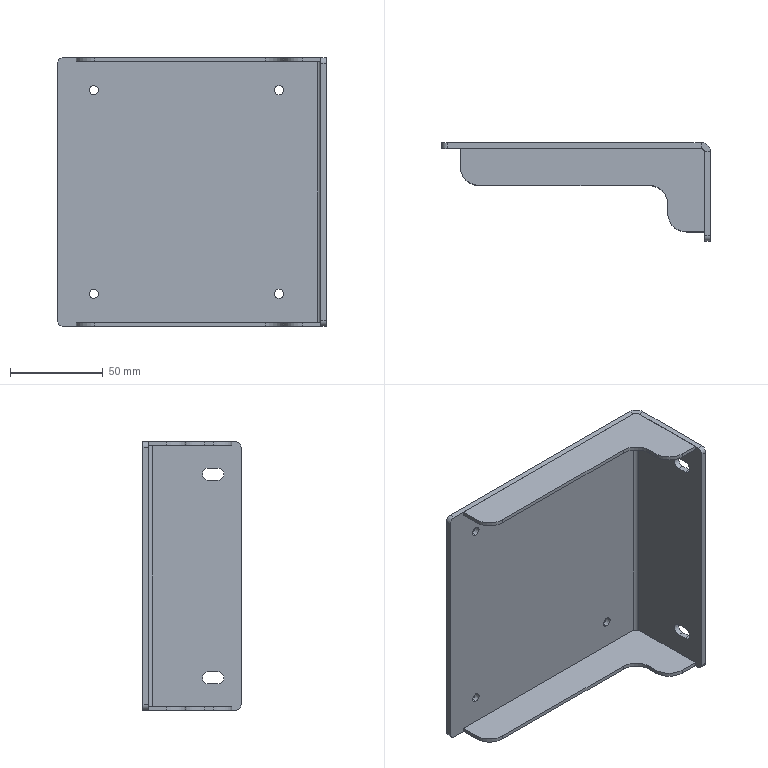Part | SolidWorks | features FlatPattern 3, HoleWzd 2, SMBaseFlange 2, SheetMetal 2, Fillet 1, MirrorSolid 1 | 3 solids | 58 faces | box 145 x 53 x 145 mm | volume 95976 mm3 | plane 34 | cylinder 24 | commonest cylinder face diameters 5 x8 20 x6 6 x4 6.6 x4 4 x1 10 x1